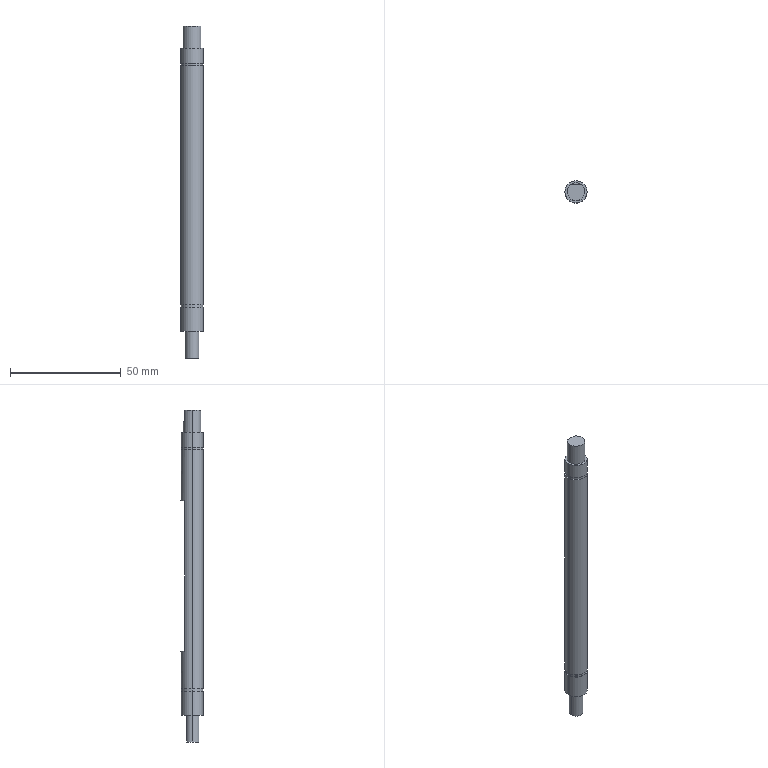Part | SolidWorks | features ICE 4, LibraryFeature 2, RevCut 2, Cut 1, Extrusion 1 | 1 solid | 29 faces | box 10 x 10 x 150 mm | volume 10228 mm3 | cylinder 15 | plane 14 | commonest cylinder face diameters 10 x6 9.6 x4 6.25 x3 8 x2
STEP:
#1=CARTESIAN_POINT('',(5.,0.,65.));
#2=VERTEX_POINT('',#1);
#3=CARTESIAN_POINT('',(-5.,0.,65.));
#4=VERTEX_POINT('',#3);
#5=CARTESIAN_POINT('',(0.,0.,65.));
#6=DIRECTION('',(0.,0.,1.));
#7=DIRECTION('',(1.,0.,0.));
#8=AXIS2_PLACEMENT_3D('',#5,#6,#7);
#9=CIRCLE('',#8,5.);
#10=EDGE_CURVE('',#2,#4,#9,.T.);
#11=ORIENTED_EDGE('',*,*,#10,.F.);
#12=CARTESIAN_POINT('',(5.,0.,58.1));
#13=VERTEX_POINT('',#12);
#14=CARTESIAN_POINT('',(5.,0.,75.));
#15=DIRECTION('',(0.,0.,-1.));
#16=VECTOR('',#15,1000.);
#17=LINE('',#14,#16);
#18=EDGE_CURVE('',#2,#13,#17,.T.);
#19=ORIENTED_EDGE('',*,*,#18,.T.);
#20=CARTESIAN_POINT('',(-5.,0.,58.1));
#21=VERTEX_POINT('',#20);
#22=CARTESIAN_POINT('',(0.,0.,58.1));
#23=DIRECTION('',(0.,0.,1.));
#24=DIRECTION('',(1.,0.,0.));
#25=AXIS2_PLACEMENT_3D('',#22,#23,#24);
#26=CIRCLE('',#25,5.);
#27=EDGE_CURVE('',#13,#21,#26,.T.);
#28=ORIENTED_EDGE('',*,*,#27,.T.);
#29=CARTESIAN_POINT('',(-5.,0.,75.));
#30=DIRECTION('',(0.,0.,-1.));
#31=VECTOR('',#30,1000.);
#32=LINE('',#29,#31);
#33=EDGE_CURVE('',#4,#21,#32,.T.);
#34=ORIENTED_EDGE('',*,*,#33,.F.);
#35=EDGE_LOOP('',(#11,#19,#28,#34));
#36=FACE_OUTER_BOUND('',#35,.T.);
#37=CARTESIAN_POINT('',(0.,0.,75.));
#38=DIRECTION('',(0.,0.,-1.));
#39=DIRECTION('',(-1.,0.,0.));
#40=AXIS2_PLACEMENT_3D('',#37,#38,#39);
#41=CYLINDRICAL_SURFACE('',#40,5.);
#42=ADVANCED_FACE('',(#36),#41,.T.);
#43=CARTESIAN_POINT('',(4.,0.,65.));
#44=VERTEX_POINT('',#43);
#45=CARTESIAN_POINT('',(-4.,0.,65.));
#46=VERTEX_POINT('',#45);
#47=CARTESIAN_POINT('',(0.,0.,65.));
#48=DIRECTION('',(0.,0.,1.));
#49=DIRECTION('',(1.,0.,0.));
#50=AXIS2_PLACEMENT_3D('',#47,#48,#49);
#51=CIRCLE('',#50,4.);
#52=EDGE_CURVE('',#44,#46,#51,.T.);
#53=ORIENTED_EDGE('',*,*,#52,.T.);
#54=CARTESIAN_POINT('',(-4.,0.,75.));
#55=VERTEX_POINT('',#54);
#56=CARTESIAN_POINT('',(-4.,0.,65.));
#57=DIRECTION('',(0.,0.,1.));
#58=VECTOR('',#57,1000.);
#59=LINE('',#56,#58);
#60=EDGE_CURVE('',#46,#55,#59,.T.);
#61=ORIENTED_EDGE('',*,*,#60,.T.);
#62=CARTESIAN_POINT('',(-2.169,3.361,75.));
#63=VERTEX_POINT('',#62);
#64=CARTESIAN_POINT('',(0.,0.,75.));
#65=DIRECTION('',(0.,0.,1.));
#66=DIRECTION('',(1.,0.,0.));
#67=AXIS2_PLACEMENT_3D('',#64,#65,#66);
#68=CIRCLE('',#67,4.);
#69=EDGE_CURVE('',#63,#55,#68,.T.);
#70=ORIENTED_EDGE('',*,*,#69,.F.);
#71=CARTESIAN_POINT('',(-2.169,3.361,70.));
#72=VERTEX_POINT('',#71);
#73=CARTESIAN_POINT('',(-2.169,3.361,65.));
#74=DIRECTION('',(0.,0.,1.));
#75=VECTOR('',#74,1000.);
#76=LINE('',#73,#75);
#77=EDGE_CURVE('',#72,#63,#76,.T.);
#78=ORIENTED_EDGE('',*,*,#77,.F.);
#79=CARTESIAN_POINT('',(2.169,3.361,70.));
#80=VERTEX_POINT('',#79);
#81=CARTESIAN_POINT('',(0.,0.,70.));
#82=DIRECTION('',(0.,0.,-1.));
#83=DIRECTION('',(1.,0.,0.));
#84=AXIS2_PLACEMENT_3D('',#81,#82,#83);
#85=CIRCLE('',#84,4.);
#86=EDGE_CURVE('',#72,#80,#85,.T.);
#87=ORIENTED_EDGE('',*,*,#86,.T.);
#88=CARTESIAN_POINT('',(2.169,3.361,75.));
#89=VERTEX_POINT('',#88);
#90=CARTESIAN_POINT('',(2.169,3.361,65.));
#91=DIRECTION('',(0.,0.,-1.));
#92=VECTOR('',#91,1000.);
#93=LINE('',#90,#92);
#94=EDGE_CURVE('',#89,#80,#93,.T.);
#95=ORIENTED_EDGE('',*,*,#94,.F.);
#96=CARTESIAN_POINT('',(4.,0.,75.));
#97=VERTEX_POINT('',#96);
#98=CARTESIAN_POINT('',(0.,0.,75.));
#99=DIRECTION('',(0.,0.,1.));
#100=DIRECTION('',(1.,0.,0.));
#101=AXIS2_PLACEMENT_3D('',#98,#99,#100);
#102=CIRCLE('',#101,4.);
#103=EDGE_CURVE('',#97,#89,#102,.T.);
#104=ORIENTED_EDGE('',*,*,#103,.F.);
#105=CARTESIAN_POINT('',(4.,0.,65.));
#106=DIRECTION('',(0.,0.,1.));
#107=VECTOR('',#106,1000.);
#108=LINE('',#105,#107);
#109=EDGE_CURVE('',#44,#97,#108,.T.);
#110=ORIENTED_EDGE('',*,*,#109,.F.);
#111=EDGE_LOOP('',(#53,#61,#70,#78,#87,#95,#104,#110));
#112=FACE_OUTER_BOUND('',#111,.T.);
#113=CARTESIAN_POINT('',(0.,0.,65.));
#114=DIRECTION('',(0.,0.,1.));
#115=DIRECTION('',(1.,0.,0.));
#116=AXIS2_PLACEMENT_3D('',#113,#114,#115);
#117=CYLINDRICAL_SURFACE('',#116,4.);
#118=ADVANCED_FACE('',(#112),#117,.T.);
#119=CARTESIAN_POINT('',(4.8,0.,57.));
#120=VERTEX_POINT('',#119);
#121=CARTESIAN_POINT('',(-4.8,0.,57.));
#122=VERTEX_POINT('',#121);
#123=CARTESIAN_POINT('',(0.,0.,57.));
#124=DIRECTION('',(0.,0.,1.));
#125=DIRECTION('',(1.,0.,0.));
#126=AXIS2_PLACEMENT_3D('',#123,#124,#125);
#127=CIRCLE('',#126,4.8);
#128=EDGE_CURVE('',#120,#122,#127,.T.);
#129=ORIENTED_EDGE('',*,*,#128,.T.);
#130=CARTESIAN_POINT('',(-4.8,0.,58.1));
#131=VERTEX_POINT('',#130);
#132=CARTESIAN_POINT('',(-4.8,0.,65.));
#133=DIRECTION('',(0.,0.,1.));
#134=VECTOR('',#133,1000.);
#135=LINE('',#132,#134);
#136=EDGE_CURVE('',#122,#131,#135,.T.);
#137=ORIENTED_EDGE('',*,*,#136,.T.);
#138=CARTESIAN_POINT('',(4.8,0.,58.1));
#139=VERTEX_POINT('',#138);
#140=CARTESIAN_POINT('',(0.,0.,58.1));
#141=DIRECTION('',(0.,0.,1.));
#142=DIRECTION('',(1.,0.,0.));
#143=AXIS2_PLACEMENT_3D('',#140,#141,#142);
#144=CIRCLE('',#143,4.8);
#145=EDGE_CURVE('',#139,#131,#144,.T.);
#146=ORIENTED_EDGE('',*,*,#145,.F.);
#147=CARTESIAN_POINT('',(4.8,0.,65.));
#148=DIRECTION('',(0.,0.,1.));
#149=VECTOR('',#148,1000.);
#150=LINE('',#147,#149);
#151=EDGE_CURVE('',#120,#139,#150,.T.);
#152=ORIENTED_EDGE('',*,*,#151,.F.);
#153=EDGE_LOOP('',(#129,#137,#146,#152));
#154=FACE_OUTER_BOUND('',#153,.T.);
#155=CARTESIAN_POINT('',(0.,0.,65.));
#156=DIRECTION('',(0.,0.,1.));
#157=DIRECTION('',(1.,0.,0.));
#158=AXIS2_PLACEMENT_3D('',#155,#156,#157);
#159=CYLINDRICAL_SURFACE('',#158,4.8);
#160=ADVANCED_FACE('',(#154),#159,.T.);
#161=CARTESIAN_POINT('',(3.842,3.2,34.));
#162=VERTEX_POINT('',#161);
#163=CARTESIAN_POINT('',(-3.842,3.2,34.));
#164=VERTEX_POINT('',#163);
#165=CARTESIAN_POINT('',(0.,0.,34.));
#166=DIRECTION('',(0.,0.,1.));
#167=DIRECTION('',(1.,0.,0.));
#168=AXIS2_PLACEMENT_3D('',#165,#166,#167);
#169=CIRCLE('',#168,5.);
#170=EDGE_CURVE('',#162,#164,#169,.T.);
#171=ORIENTED_EDGE('',*,*,#170,.T.);
#172=CARTESIAN_POINT('',(-3.842,3.2,-34.));
#173=VERTEX_POINT('',#172);
#174=CARTESIAN_POINT('',(-3.842,3.2,75.));
#175=DIRECTION('',(0.,0.,-1.));
#176=VECTOR('',#175,1000.);
#177=LINE('',#174,#176);
#178=EDGE_CURVE('',#164,#173,#177,.T.);
#179=ORIENTED_EDGE('',*,*,#178,.T.);
#180=CARTESIAN_POINT('',(3.842,3.2,-34.));
#181=VERTEX_POINT('',#180);
#182=CARTESIAN_POINT('',(0.,0.,-34.));
#183=DIRECTION('',(0.,0.,-1.));
#184=DIRECTION('',(-1.,0.,0.));
#185=AXIS2_PLACEMENT_3D('',#182,#183,#184);
#186=CIRCLE('',#185,5.);
#187=EDGE_CURVE('',#173,#181,#186,.T.);
#188=ORIENTED_EDGE('',*,*,#187,.T.);
#189=CARTESIAN_POINT('',(3.842,3.2,75.));
#190=DIRECTION('',(0.,0.,1.));
#191=VECTOR('',#190,1000.);
#192=LINE('',#189,#191);
#193=EDGE_CURVE('',#181,#162,#192,.T.);
#194=ORIENTED_EDGE('',*,*,#193,.T.);
#195=EDGE_LOOP('',(#171,#179,#188,#194));
#196=FACE_BOUND('',#195,.T.);
#197=CARTESIAN_POINT('',(5.,0.,57.));
#198=VERTEX_POINT('',#197);
#199=CARTESIAN_POINT('',(-5.,0.,57.));
#200=VERTEX_POINT('',#199);
#201=CARTESIAN_POINT('',(0.,0.,57.));
#202=DIRECTION('',(0.,0.,1.));
#203=DIRECTION('',(1.,0.,0.));
#204=AXIS2_PLACEMENT_3D('',#201,#202,#203);
#205=CIRCLE('',#204,5.);
#206=EDGE_CURVE('',#198,#200,#205,.T.);
#207=ORIENTED_EDGE('',*,*,#206,.F.);
#208=CARTESIAN_POINT('',(5.,0.,-51.));
#209=VERTEX_POINT('',#208);
#210=CARTESIAN_POINT('',(5.,0.,75.));
#211=DIRECTION('',(0.,0.,-1.));
#212=VECTOR('',#211,1000.);
#213=LINE('',#210,#212);
#214=EDGE_CURVE('',#198,#209,#213,.T.);
#215=ORIENTED_EDGE('',*,*,#214,.T.);
#216=CARTESIAN_POINT('',(-5.,0.,-51.));
#217=VERTEX_POINT('',#216);
#218=CARTESIAN_POINT('',(0.,0.,-51.));
#219=DIRECTION('',(0.,0.,-1.));
#220=DIRECTION('',(-1.,0.,0.));
#221=AXIS2_PLACEMENT_3D('',#218,#219,#220);
#222=CIRCLE('',#221,5.);
#223=EDGE_CURVE('',#217,#209,#222,.T.);
#224=ORIENTED_EDGE('',*,*,#223,.F.);
#225=CARTESIAN_POINT('',(-5.,0.,75.));
#226=DIRECTION('',(0.,0.,-1.));
#227=VECTOR('',#226,1000.);
#228=LINE('',#225,#227);
#229=EDGE_CURVE('',#200,#217,#228,.T.);
#230=ORIENTED_EDGE('',*,*,#229,.F.);
#231=EDGE_LOOP('',(#207,#215,#224,#230));
#232=FACE_OUTER_BOUND('',#231,.T.);
#233=CARTESIAN_POINT('',(0.,0.,75.));
#234=DIRECTION('',(0.,0.,-1.));
#235=DIRECTION('',(-1.,0.,0.));
#236=AXIS2_PLACEMENT_3D('',#233,#234,#235);
#237=CYLINDRICAL_SURFACE('',#236,5.);
#238=ADVANCED_FACE('',(#196,#232),#237,.T.);
#239=CARTESIAN_POINT('',(-4.8,0.,-51.));
#240=VERTEX_POINT('',#239);
#241=CARTESIAN_POINT('',(4.8,0.,-51.));
#242=VERTEX_POINT('',#241);
#243=CARTESIAN_POINT('',(0.,0.,-51.));
#244=DIRECTION('',(0.,0.,-1.));
#245=DIRECTION('',(-1.,0.,0.));
#246=AXIS2_PLACEMENT_3D('',#243,#244,#245);
#247=CIRCLE('',#246,4.8);
#248=EDGE_CURVE('',#240,#242,#247,.T.);
#249=ORIENTED_EDGE('',*,*,#248,.T.);
#250=CARTESIAN_POINT('',(4.8,0.,-52.1));
#251=VERTEX_POINT('',#250);
#252=CARTESIAN_POINT('',(4.8,0.,-63.));
#253=DIRECTION('',(0.,0.,-1.));
#254=VECTOR('',#253,1000.);
#255=LINE('',#252,#254);
#256=EDGE_CURVE('',#242,#251,#255,.T.);
#257=ORIENTED_EDGE('',*,*,#256,.T.);
#258=CARTESIAN_POINT('',(-4.8,0.,-52.1));
#259=VERTEX_POINT('',#258);
#260=CARTESIAN_POINT('',(0.,0.,-52.1));
#261=DIRECTION('',(0.,0.,-1.));
#262=DIRECTION('',(-1.,0.,0.));
#263=AXIS2_PLACEMENT_3D('',#260,#261,#262);
#264=CIRCLE('',#263,4.8);
#265=EDGE_CURVE('',#259,#251,#264,.T.);
#266=ORIENTED_EDGE('',*,*,#265,.F.);
#267=CARTESIAN_POINT('',(-4.8,0.,-63.));
#268=DIRECTION('',(0.,0.,-1.));
#269=VECTOR('',#268,1000.);
#270=LINE('',#267,#269);
#271=EDGE_CURVE('',#240,#259,#270,.T.);
#272=ORIENTED_EDGE('',*,*,#271,.F.);
#273=EDGE_LOOP('',(#249,#257,#266,#272));
#274=FACE_OUTER_BOUND('',#273,.T.);
#275=CARTESIAN_POINT('',(0.,0.,-63.));
#276=DIRECTION('',(0.,0.,-1.));
#277=DIRECTION('',(-1.,0.,0.));
#278=AXIS2_PLACEMENT_3D('',#275,#276,#277);
#279=CYLINDRICAL_SURFACE('',#278,4.8);
#280=ADVANCED_FACE('',(#274),#279,.T.);
#281=CARTESIAN_POINT('',(1.875,2.5,-63.));
#282=VERTEX_POINT('',#281);
#283=CARTESIAN_POINT('',(3.125,0.,-63.));
#284=VERTEX_POINT('',#283);
#285=CARTESIAN_POINT('',(0.,0.,-63.));
#286=DIRECTION('',(0.,0.,-1.));
#287=DIRECTION('',(-1.,0.,0.));
#288=AXIS2_PLACEMENT_3D('',#285,#286,#287);
#289=CIRCLE('',#288,3.125);
#290=EDGE_CURVE('',#282,#284,#289,.T.);
#291=ORIENTED_EDGE('',*,*,#290,.T.);
#292=CARTESIAN_POINT('',(3.125,0.,-75.));
#293=VERTEX_POINT('',#292);
#294=CARTESIAN_POINT('',(3.125,0.,-63.));
#295=DIRECTION('',(0.,0.,-1.));
#296=VECTOR('',#295,1000.);
#297=LINE('',#294,#296);
#298=EDGE_CURVE('',#284,#293,#297,.T.);
#299=ORIENTED_EDGE('',*,*,#298,.T.);
#300=CARTESIAN_POINT('',(1.875,2.5,-75.));
#301=VERTEX_POINT('',#300);
#302=CARTESIAN_POINT('',(0.,0.,-75.));
#303=DIRECTION('',(0.,0.,-1.));
#304=DIRECTION('',(-1.,0.,0.));
#305=AXIS2_PLACEMENT_3D('',#302,#303,#304);
#306=CIRCLE('',#305,3.125);
#307=EDGE_CURVE('',#301,#293,#306,.T.);
#308=ORIENTED_EDGE('',*,*,#307,.F.);
#309=CARTESIAN_POINT('',(1.875,2.5,-63.));
#310=DIRECTION('',(0.,0.,1.));
#311=VECTOR('',#310,1000.);
#312=LINE('',#309,#311);
#313=EDGE_CURVE('',#301,#282,#312,.T.);
#314=ORIENTED_EDGE('',*,*,#313,.T.);
#315=EDGE_LOOP('',(#291,#299,#308,#314));
#316=FACE_OUTER_BOUND('',#315,.T.);
#317=CARTESIAN_POINT('',(0.,0.,-63.));
#318=DIRECTION('',(0.,0.,-1.));
#319=DIRECTION('',(-1.,0.,0.));
#320=AXIS2_PLACEMENT_3D('',#317,#318,#319);
#321=CYLINDRICAL_SURFACE('',#320,3.125);
#322=ADVANCED_FACE('',(#316),#321,.T.);
#323=ORIENTED_EDGE('',*,*,#298,.F.);
#324=CARTESIAN_POINT('',(-3.125,0.,-63.));
#325=VERTEX_POINT('',#324);
#326=CARTESIAN_POINT('',(0.,0.,-63.));
#327=DIRECTION('',(0.,0.,-1.));
#328=DIRECTION('',(-1.,0.,0.));
#329=AXIS2_PLACEMENT_3D('',#326,#327,#328);
#330=CIRCLE('',#329,3.125);
#331=EDGE_CURVE('',#284,#325,#330,.T.);
#332=ORIENTED_EDGE('',*,*,#331,.T.);
#333=CARTESIAN_POINT('',(-3.125,0.,-75.));
#334=VERTEX_POINT('',#333);
#335=CARTESIAN_POINT('',(-3.125,0.,-63.));
#336=DIRECTION('',(0.,0.,-1.));
#337=VECTOR('',#336,1000.);
#338=LINE('',#335,#337);
#339=EDGE_CURVE('',#325,#334,#338,.T.);
#340=ORIENTED_EDGE('',*,*,#339,.T.);
#341=CARTESIAN_POINT('',(0.,0.,-75.));
#342=DIRECTION('',(0.,0.,-1.));
#343=DIRECTION('',(-1.,0.,0.));
#344=AXIS2_PLACEMENT_3D('',#341,#342,#343);
#345=CIRCLE('',#344,3.125);
#346=EDGE_CURVE('',#293,#334,#345,.T.);
#347=ORIENTED_EDGE('',*,*,#346,.F.);
#348=EDGE_LOOP('',(#323,#332,#340,#347));
#349=FACE_OUTER_BOUND('',#348,.T.);
#350=CARTESIAN_POINT('',(0.,0.,-63.));
#351=DIRECTION('',(0.,0.,-1.));
#352=DIRECTION('',(-1.,0.,0.));
#353=AXIS2_PLACEMENT_3D('',#350,#351,#352);
#354=CYLINDRICAL_SURFACE('',#353,3.125);
#355=ADVANCED_FACE('',(#349),#354,.T.);
#356=CARTESIAN_POINT('',(-5.,0.,-52.1));
#357=VERTEX_POINT('',#356);
#358=CARTESIAN_POINT('',(5.,0.,-52.1));
#359=VERTEX_POINT('',#358);
#360=CARTESIAN_POINT('',(0.,0.,-52.1));
#361=DIRECTION('',(0.,0.,-1.));
#362=DIRECTION('',(-1.,0.,0.));
#363=AXIS2_PLACEMENT_3D('',#360,#361,#362);
#364=CIRCLE('',#363,5.);
#365=EDGE_CURVE('',#357,#359,#364,.T.);
#366=ORIENTED_EDGE('',*,*,#365,.T.);
#367=CARTESIAN_POINT('',(5.,0.,-63.));
#368=VERTEX_POINT('',#367);
#369=CARTESIAN_POINT('',(5.,0.,75.));
#370=DIRECTION('',(0.,0.,-1.));
#371=VECTOR('',#370,1000.);
#372=LINE('',#369,#371);
#373=EDGE_CURVE('',#359,#368,#372,.T.);
#374=ORIENTED_EDGE('',*,*,#373,.T.);
#375=CARTESIAN_POINT('',(-5.,0.,-63.));
#376=VERTEX_POINT('',#375);
#377=CARTESIAN_POINT('',(0.,0.,-63.));
#378=DIRECTION('',(0.,0.,-1.));
#379=DIRECTION('',(-1.,0.,0.));
#380=AXIS2_PLACEMENT_3D('',#377,#378,#379);
#381=CIRCLE('',#380,5.);
#382=EDGE_CURVE('',#376,#368,#381,.T.);
#383=ORIENTED_EDGE('',*,*,#382,.F.);
#384=CARTESIAN_POINT('',(-5.,0.,75.));
#385=DIRECTION('',(0.,0.,-1.));
#386=VECTOR('',#385,1000.);
#387=LINE('',#384,#386);
#388=EDGE_CURVE('',#357,#376,#387,.T.);
#389=ORIENTED_EDGE('',*,*,#388,.F.);
#390=EDGE_LOOP('',(#366,#374,#383,#389));
#391=FACE_OUTER_BOUND('',#390,.T.);
#392=CARTESIAN_POINT('',(0.,0.,75.));
#393=DIRECTION('',(0.,0.,-1.));
#394=DIRECTION('',(-1.,0.,0.));
#395=AXIS2_PLACEMENT_3D('',#392,#393,#394);
#396=CYLINDRICAL_SURFACE('',#395,5.);
#397=ADVANCED_FACE('',(#391),#396,.T.);
#398=ORIENTED_EDGE('',*,*,#373,.F.);
#399=CARTESIAN_POINT('',(0.,0.,-52.1));
#400=DIRECTION('',(0.,0.,-1.));
#401=DIRECTION('',(-1.,0.,0.));
#402=AXIS2_PLACEMENT_3D('',#399,#400,#401);
#403=CIRCLE('',#402,5.);
#404=EDGE_CURVE('',#359,#357,#403,.T.);
#405=ORIENTED_EDGE('',*,*,#404,.T.);
#406=ORIENTED_EDGE('',*,*,#388,.T.);
#407=CARTESIAN_POINT('',(0.,0.,-63.));
#408=DIRECTION('',(0.,0.,-1.));
#409=DIRECTION('',(-1.,0.,0.));
#410=AXIS2_PLACEMENT_3D('',#407,#408,#409);
#411=CIRCLE('',#410,5.);
#412=EDGE_CURVE('',#368,#376,#411,.T.);
#413=ORIENTED_EDGE('',*,*,#412,.F.);
#414=EDGE_LOOP('',(#398,#405,#406,#413));
#415=FACE_OUTER_BOUND('',#414,.T.);
#416=CARTESIAN_POINT('',(0.,0.,75.));
#417=DIRECTION('',(0.,0.,-1.));
#418=DIRECTION('',(-1.,0.,0.));
#419=AXIS2_PLACEMENT_3D('',#416,#417,#418);
#420=CYLINDRICAL_SURFACE('',#419,5.);
#421=ADVANCED_FACE('',(#415),#420,.T.);
#422=ORIENTED_EDGE('',*,*,#339,.F.);
#423=CARTESIAN_POINT('',(-1.875,2.5,-63.));
#424=VERTEX_POINT('',#423);
#425=CARTESIAN_POINT('',(0.,0.,-63.));
#426=DIRECTION('',(0.,0.,-1.));
#427=DIRECTION('',(-1.,0.,0.));
#428=AXIS2_PLACEMENT_3D('',#425,#426,#427);
#429=CIRCLE('',#428,3.125);
#430=EDGE_CURVE('',#325,#424,#429,.T.);
#431=ORIENTED_EDGE('',*,*,#430,.T.);
#432=CARTESIAN_POINT('',(-1.875,2.5,-75.));
#433=VERTEX_POINT('',#432);
#434=CARTESIAN_POINT('',(-1.875,2.5,-63.));
#435=DIRECTION('',(0.,0.,-1.));
#436=VECTOR('',#435,1000.);
#437=LINE('',#434,#436);
#438=EDGE_CURVE('',#424,#433,#437,.T.);
#439=ORIENTED_EDGE('',*,*,#438,.T.);
#440=CARTESIAN_POINT('',(0.,0.,-75.));
#441=DIRECTION('',(0.,0.,-1.));
#442=DIRECTION('',(-1.,0.,0.));
#443=AXIS2_PLACEMENT_3D('',#440,#441,#442);
#444=CIRCLE('',#443,3.125);
#445=EDGE_CURVE('',#334,#433,#444,.T.);
#446=ORIENTED_EDGE('',*,*,#445,.F.);
#447=EDGE_LOOP('',(#422,#431,#439,#446));
#448=FACE_OUTER_BOUND('',#447,.T.);
#449=CARTESIAN_POINT('',(0.,0.,-63.));
#450=DIRECTION('',(0.,0.,-1.));
#451=DIRECTION('',(-1.,0.,0.));
#452=AXIS2_PLACEMENT_3D('',#449,#450,#451);
#453=CYLINDRICAL_SURFACE('',#452,3.125);
#454=ADVANCED_FACE('',(#448),#453,.T.);
#455=CARTESIAN_POINT('',(0.,2.5,-75.));
#456=DIRECTION('',(-1.,0.,0.));
#457=VECTOR('',#456,1000.);
#458=LINE('',#455,#457);
#459=EDGE_CURVE('',#301,#433,#458,.T.);
#460=ORIENTED_EDGE('',*,*,#459,.F.);
#461=ORIENTED_EDGE('',*,*,#307,.T.);
#462=ORIENTED_EDGE('',*,*,#346,.T.);
#463=ORIENTED_EDGE('',*,*,#445,.T.);
#464=EDGE_LOOP('',(#460,#461,#462,#463));
#465=FACE_OUTER_BOUND('',#464,.T.);
#466=CARTESIAN_POINT('',(0.,0.,-75.));
#467=DIRECTION('',(0.,0.,1.));
#468=DIRECTION('',(1.,0.,0.));
#469=AXIS2_PLACEMENT_3D('',#466,#467,#468);
#470=PLANE('',#469);
#471=ADVANCED_FACE('',(#465),#470,.F.);
#472=CARTESIAN_POINT('',(1.957,2.5,-63.));
#473=DIRECTION('',(1.,0.,0.));
#474=VECTOR('',#473,1000.);
#475=LINE('',#472,#474);
#476=EDGE_CURVE('',#424,#282,#475,.T.);
#477=ORIENTED_EDGE('',*,*,#476,.F.);
#478=ORIENTED_EDGE('',*,*,#430,.F.);
#479=ORIENTED_EDGE('',*,*,#331,.F.);
#480=ORIENTED_EDGE('',*,*,#290,.F.);
#481=EDGE_LOOP('',(#477,#478,#479,#480));
#482=FACE_BOUND('',#481,.T.);
#483=ORIENTED_EDGE('',*,*,#382,.T.);
#484=ORIENTED_EDGE('',*,*,#412,.T.);
#485=EDGE_LOOP('',(#483,#484));
#486=FACE_OUTER_BOUND('',#485,.T.);
#487=CARTESIAN_POINT('',(0.,0.,-63.));
#488=DIRECTION('',(0.,0.,-1.));
#489=DIRECTION('',(-1.,0.,0.));
#490=AXIS2_PLACEMENT_3D('',#487,#488,#489);
#491=PLANE('',#490);
#492=ADVANCED_FACE('',(#482,#486),#491,.T.);
#493=ORIENTED_EDGE('',*,*,#459,.T.);
#494=ORIENTED_EDGE('',*,*,#438,.F.);
#495=ORIENTED_EDGE('',*,*,#476,.T.);
#496=ORIENTED_EDGE('',*,*,#313,.F.);
#497=EDGE_LOOP('',(#493,#494,#495,#496));
#498=FACE_OUTER_BOUND('',#497,.T.);
#499=CARTESIAN_POINT('',(1.957,2.5,-63.));
#500=DIRECTION('',(0.,1.,0.));
#501=DIRECTION('',(0.,0.,1.));
#502=AXIS2_PLACEMENT_3D('',#499,#500,#501);
#503=PLANE('',#502);
#504=ADVANCED_FACE('',(#498),#503,.T.);
#505=ORIENTED_EDGE('',*,*,#365,.F.);
#506=ORIENTED_EDGE('',*,*,#404,.F.);
#507=EDGE_LOOP('',(#505,#506));
#508=FACE_OUTER_BOUND('',#507,.T.);
#509=ORIENTED_EDGE('',*,*,#265,.T.);
#510=CARTESIAN_POINT('',(0.,0.,-52.1));
#511=DIRECTION('',(0.,0.,-1.));
#512=DIRECTION('',(-1.,0.,0.));
#513=AXIS2_PLACEMENT_3D('',#510,#511,#512);
#514=CIRCLE('',#513,4.8);
#515=EDGE_CURVE('',#251,#259,#514,.T.);
#516=ORIENTED_EDGE('',*,*,#515,.T.);
#517=EDGE_LOOP('',(#509,#516));
#518=FACE_BOUND('',#517,.T.);
#519=CARTESIAN_POINT('',(-5.,0.,-52.1));
#520=DIRECTION('',(0.,0.,-1.));
#521=DIRECTION('',(-1.,0.,0.));
#522=AXIS2_PLACEMENT_3D('',#519,#520,#521);
#523=PLANE('',#522);
#524=ADVANCED_FACE('',(#508,#518),#523,.F.);
#525=ORIENTED_EDGE('',*,*,#256,.F.);
#526=CARTESIAN_POINT('',(0.,0.,-51.));
#527=DIRECTION('',(0.,0.,-1.));
#528=DIRECTION('',(-1.,0.,0.));
#529=AXIS2_PLACEMENT_3D('',#526,#527,#528);
#530=CIRCLE('',#529,4.8);
#531=EDGE_CURVE('',#242,#240,#530,.T.);
#532=ORIENTED_EDGE('',*,*,#531,.T.);
#533=ORIENTED_EDGE('',*,*,#271,.T.);
#534=ORIENTED_EDGE('',*,*,#515,.F.);
#535=EDGE_LOOP('',(#525,#532,#533,#534));
#536=FACE_OUTER_BOUND('',#535,.T.);
#537=CARTESIAN_POINT('',(0.,0.,-63.));
#538=DIRECTION('',(0.,0.,-1.));
#539=DIRECTION('',(-1.,0.,0.));
#540=AXIS2_PLACEMENT_3D('',#537,#538,#539);
#541=CYLINDRICAL_SURFACE('',#540,4.8);
#542=ADVANCED_FACE('',(#536),#541,.T.);
#543=ORIENTED_EDGE('',*,*,#248,.F.);
#544=ORIENTED_EDGE('',*,*,#531,.F.);
#545=EDGE_LOOP('',(#543,#544));
#546=FACE_BOUND('',#545,.T.);
#547=ORIENTED_EDGE('',*,*,#223,.T.);
#548=CARTESIAN_POINT('',(0.,0.,-51.));
#549=DIRECTION('',(0.,0.,-1.));
#550=DIRECTION('',(-1.,0.,0.));
#551=AXIS2_PLACEMENT_3D('',#548,#549,#550);
#552=CIRCLE('',#551,5.);
#553=EDGE_CURVE('',#209,#217,#552,.T.);
#554=ORIENTED_EDGE('',*,*,#553,.T.);
#555=EDGE_LOOP('',(#547,#554));
#556=FACE_OUTER_BOUND('',#555,.T.);
#557=CARTESIAN_POINT('',(-5.,0.,-51.));
#558=DIRECTION('',(0.,0.,1.));
#559=DIRECTION('',(1.,0.,0.));
#560=AXIS2_PLACEMENT_3D('',#557,#558,#559);
#561=PLANE('',#560);
#562=ADVANCED_FACE('',(#546,#556),#561,.F.);
#563=CARTESIAN_POINT('',(-5.,3.2,-34.));
#564=DIRECTION('',(1.,0.,0.));
#565=VECTOR('',#564,1000.);
#566=LINE('',#563,#565);
#567=EDGE_CURVE('',#173,#181,#566,.T.);
#568=ORIENTED_EDGE('',*,*,#567,.T.);
#569=ORIENTED_EDGE('',*,*,#187,.F.);
#570=EDGE_LOOP('',(#568,#569));
#571=FACE_OUTER_BOUND('',#570,.T.);
#572=CARTESIAN_POINT('',(-5.,17.735,-34.));
#573=DIRECTION('',(0.,0.,-1.));
#574=DIRECTION('',(-1.,0.,0.));
#575=AXIS2_PLACEMENT_3D('',#572,#573,#574);
#576=PLANE('',#575);
#577=ADVANCED_FACE('',(#571),#576,.F.);
#578=CARTESIAN_POINT('',(-5.,3.2,34.));
#579=DIRECTION('',(1.,0.,0.));
#580=VECTOR('',#579,1000.);
#581=LINE('',#578,#580);
#582=EDGE_CURVE('',#164,#162,#581,.T.);
#583=ORIENTED_EDGE('',*,*,#582,.T.);
#584=ORIENTED_EDGE('',*,*,#193,.F.);
#585=ORIENTED_EDGE('',*,*,#567,.F.);
#586=ORIENTED_EDGE('',*,*,#178,.F.);
#587=EDGE_LOOP('',(#583,#584,#585,#586));
#588=FACE_OUTER_BOUND('',#587,.T.);
#589=CARTESIAN_POINT('',(-5.,3.2,34.));
#590=DIRECTION('',(0.,-1.,0.));
#591=DIRECTION('',(0.,0.,-1.));
#592=AXIS2_PLACEMENT_3D('',#589,#590,#591);
#593=PLANE('',#592);
#594=ADVANCED_FACE('',(#588),#593,.F.);
#595=ORIENTED_EDGE('',*,*,#582,.F.);
#596=ORIENTED_EDGE('',*,*,#170,.F.);
#597=EDGE_LOOP('',(#595,#596));
#598=FACE_OUTER_BOUND('',#597,.T.);
#599=CARTESIAN_POINT('',(-5.,17.735,34.));
#600=DIRECTION('',(0.,0.,1.));
#601=DIRECTION('',(1.,0.,0.));
#602=AXIS2_PLACEMENT_3D('',#599,#600,#601);
#603=PLANE('',#602);
#604=ADVANCED_FACE('',(#598),#603,.F.);
#605=ORIENTED_EDGE('',*,*,#214,.F.);
#606=CARTESIAN_POINT('',(0.,0.,57.));
#607=DIRECTION('',(0.,0.,1.));
#608=DIRECTION('',(1.,0.,0.));
#609=AXIS2_PLACEMENT_3D('',#606,#607,#608);
#610=CIRCLE('',#609,5.);
#611=EDGE_CURVE('',#200,#198,#610,.T.);
#612=ORIENTED_EDGE('',*,*,#611,.F.);
#613=ORIENTED_EDGE('',*,*,#229,.T.);
#614=ORIENTED_EDGE('',*,*,#553,.F.);
#615=EDGE_LOOP('',(#605,#612,#613,#614));
#616=FACE_OUTER_BOUND('',#615,.T.);
#617=CARTESIAN_POINT('',(0.,0.,75.));
#618=DIRECTION('',(0.,0.,-1.));
#619=DIRECTION('',(-1.,0.,0.));
#620=AXIS2_PLACEMENT_3D('',#617,#618,#619);
#621=CYLINDRICAL_SURFACE('',#620,5.);
#622=ADVANCED_FACE('',(#616),#621,.T.);
#623=CARTESIAN_POINT('',(0.,0.,58.1));
#624=DIRECTION('',(0.,0.,1.));
#625=DIRECTION('',(1.,0.,0.));
#626=AXIS2_PLACEMENT_3D('',#623,#624,#625);
#627=CIRCLE('',#626,5.);
#628=EDGE_CURVE('',#21,#13,#627,.T.);
#629=ORIENTED_EDGE('',*,*,#628,.F.);
#630=ORIENTED_EDGE('',*,*,#27,.F.);
#631=EDGE_LOOP('',(#629,#630));
#632=FACE_OUTER_BOUND('',#631,.T.);
#633=ORIENTED_EDGE('',*,*,#145,.T.);
#634=CARTESIAN_POINT('',(0.,0.,58.1));
#635=DIRECTION('',(0.,0.,1.));
#636=DIRECTION('',(1.,0.,0.));
#637=AXIS2_PLACEMENT_3D('',#634,#635,#636);
#638=CIRCLE('',#637,4.8);
#639=EDGE_CURVE('',#131,#139,#638,.T.);
#640=ORIENTED_EDGE('',*,*,#639,.T.);
#641=EDGE_LOOP('',(#633,#640));
#642=FACE_BOUND('',#641,.T.);
#643=CARTESIAN_POINT('',(5.,0.,58.1));
#644=DIRECTION('',(0.,0.,1.));
#645=DIRECTION('',(1.,0.,0.));
#646=AXIS2_PLACEMENT_3D('',#643,#644,#645);
#647=PLANE('',#646);
#648=ADVANCED_FACE('',(#632,#642),#647,.F.);
#649=ORIENTED_EDGE('',*,*,#136,.F.);
#650=CARTESIAN_POINT('',(0.,0.,57.));
#651=DIRECTION('',(0.,0.,1.));
#652=DIRECTION('',(1.,0.,0.));
#653=AXIS2_PLACEMENT_3D('',#650,#651,#652);
#654=CIRCLE('',#653,4.8);
#655=EDGE_CURVE('',#122,#120,#654,.T.);
#656=ORIENTED_EDGE('',*,*,#655,.T.);
#657=ORIENTED_EDGE('',*,*,#151,.T.);
#658=ORIENTED_EDGE('',*,*,#639,.F.);
#659=EDGE_LOOP('',(#649,#656,#657,#658));
#660=FACE_OUTER_BOUND('',#659,.T.);
#661=CARTESIAN_POINT('',(0.,0.,65.));
#662=DIRECTION('',(0.,0.,1.));
#663=DIRECTION('',(1.,0.,0.));
#664=AXIS2_PLACEMENT_3D('',#661,#662,#663);
#665=CYLINDRICAL_SURFACE('',#664,4.8);
#666=ADVANCED_FACE('',(#660),#665,.T.);
#667=ORIENTED_EDGE('',*,*,#128,.F.);
#668=ORIENTED_EDGE('',*,*,#655,.F.);
#669=EDGE_LOOP('',(#667,#668));
#670=FACE_BOUND('',#669,.T.);
#671=ORIENTED_EDGE('',*,*,#611,.T.);
#672=ORIENTED_EDGE('',*,*,#206,.T.);
#673=EDGE_LOOP('',(#671,#672));
#674=FACE_OUTER_BOUND('',#673,.T.);
#675=CARTESIAN_POINT('',(5.,0.,57.));
#676=DIRECTION('',(0.,0.,-1.));
#677=DIRECTION('',(-1.,0.,0.));
#678=AXIS2_PLACEMENT_3D('',#675,#676,#677);
#679=PLANE('',#678);
#680=ADVANCED_FACE('',(#670,#674),#679,.F.);
#681=CARTESIAN_POINT('',(-5.016,3.361,70.));
#682=DIRECTION('',(1.,0.,0.));
#683=VECTOR('',#682,1000.);
#684=LINE('',#681,#683);
#685=EDGE_CURVE('',#72,#80,#684,.T.);
#686=ORIENTED_EDGE('',*,*,#685,.T.);
#687=ORIENTED_EDGE('',*,*,#86,.F.);
#688=EDGE_LOOP('',(#686,#687));
#689=FACE_OUTER_BOUND('',#688,.T.);
#690=CARTESIAN_POINT('',(0.,0.,70.));
#691=DIRECTION('',(0.,0.,1.));
#692=DIRECTION('',(1.,0.,0.));
#693=AXIS2_PLACEMENT_3D('',#690,#691,#692);
#694=PLANE('',#693);
#695=ADVANCED_FACE('',(#689),#694,.T.);
#696=CARTESIAN_POINT('',(0.,3.361,75.));
#697=DIRECTION('',(1.,0.,0.));
#698=VECTOR('',#697,1000.);
#699=LINE('',#696,#698);
#700=EDGE_CURVE('',#63,#89,#699,.T.);
#701=ORIENTED_EDGE('',*,*,#700,.F.);
#702=ORIENTED_EDGE('',*,*,#69,.T.);
#703=CARTESIAN_POINT('',(0.,0.,75.));
#704=DIRECTION('',(0.,0.,1.));
#705=DIRECTION('',(1.,0.,0.));
#706=AXIS2_PLACEMENT_3D('',#703,#704,#705);
#707=CIRCLE('',#706,4.);
#708=EDGE_CURVE('',#55,#97,#707,.T.);
#709=ORIENTED_EDGE('',*,*,#708,.T.);
#710=ORIENTED_EDGE('',*,*,#103,.T.);
#711=EDGE_LOOP('',(#701,#702,#709,#710));
#712=FACE_OUTER_BOUND('',#711,.T.);
#713=CARTESIAN_POINT('',(0.,0.,75.));
#714=DIRECTION('',(0.,0.,1.));
#715=DIRECTION('',(1.,0.,0.));
#716=AXIS2_PLACEMENT_3D('',#713,#714,#715);
#717=PLANE('',#716);
#718=ADVANCED_FACE('',(#712),#717,.T.);
#719=ORIENTED_EDGE('',*,*,#94,.T.);
#720=ORIENTED_EDGE('',*,*,#685,.F.);
#721=ORIENTED_EDGE('',*,*,#77,.T.);
#722=ORIENTED_EDGE('',*,*,#700,.T.);
#723=EDGE_LOOP('',(#719,#720,#721,#722));
#724=FACE_OUTER_BOUND('',#723,.T.);
#725=CARTESIAN_POINT('',(-5.016,3.361,70.));
#726=DIRECTION('',(0.,-1.,0.));
#727=DIRECTION('',(0.,0.,-1.));
#728=AXIS2_PLACEMENT_3D('',#725,#726,#727);
#729=PLANE('',#728);
#730=ADVANCED_FACE('',(#724),#729,.F.);
#731=ORIENTED_EDGE('',*,*,#60,.F.);
#732=CARTESIAN_POINT('',(0.,0.,65.));
#733=DIRECTION('',(0.,0.,1.));
#734=DIRECTION('',(1.,0.,0.));
#735=AXIS2_PLACEMENT_3D('',#732,#733,#734);
#736=CIRCLE('',#735,4.);
#737=EDGE_CURVE('',#46,#44,#736,.T.);
#738=ORIENTED_EDGE('',*,*,#737,.T.);
#739=ORIENTED_EDGE('',*,*,#109,.T.);
#740=ORIENTED_EDGE('',*,*,#708,.F.);
#741=EDGE_LOOP('',(#731,#738,#739,#740));
#742=FACE_OUTER_BOUND('',#741,.T.);
#743=CARTESIAN_POINT('',(0.,0.,65.));
#744=DIRECTION('',(0.,0.,1.));
#745=DIRECTION('',(1.,0.,0.));
#746=AXIS2_PLACEMENT_3D('',#743,#744,#745);
#747=CYLINDRICAL_SURFACE('',#746,4.);
#748=ADVANCED_FACE('',(#742),#747,.T.);
#749=ORIENTED_EDGE('',*,*,#52,.F.);
#750=ORIENTED_EDGE('',*,*,#737,.F.);
#751=EDGE_LOOP('',(#749,#750));
#752=FACE_BOUND('',#751,.T.);
#753=CARTESIAN_POINT('',(0.,0.,65.));
#754=DIRECTION('',(0.,0.,1.));
#755=DIRECTION('',(1.,0.,0.));
#756=AXIS2_PLACEMENT_3D('',#753,#754,#755);
#757=CIRCLE('',#756,5.);
#758=EDGE_CURVE('',#4,#2,#757,.T.);
#759=ORIENTED_EDGE('',*,*,#758,.T.);
#760=ORIENTED_EDGE('',*,*,#10,.T.);
#761=EDGE_LOOP('',(#759,#760));
#762=FACE_OUTER_BOUND('',#761,.T.);
#763=CARTESIAN_POINT('',(0.,0.,65.));
#764=DIRECTION('',(0.,0.,1.));
#765=DIRECTION('',(1.,0.,0.));
#766=AXIS2_PLACEMENT_3D('',#763,#764,#765);
#767=PLANE('',#766);
#768=ADVANCED_FACE('',(#752,#762),#767,.T.);
#769=ORIENTED_EDGE('',*,*,#18,.F.);
#770=ORIENTED_EDGE('',*,*,#758,.F.);
#771=ORIENTED_EDGE('',*,*,#33,.T.);
#772=ORIENTED_EDGE('',*,*,#628,.T.);
#773=EDGE_LOOP('',(#769,#770,#771,#772));
#774=FACE_OUTER_BOUND('',#773,.T.);
#775=CARTESIAN_POINT('',(0.,0.,75.));
#776=DIRECTION('',(0.,0.,-1.));
#777=DIRECTION('',(-1.,0.,0.));
#778=AXIS2_PLACEMENT_3D('',#775,#776,#777);
#779=CYLINDRICAL_SURFACE('',#778,5.);
#780=ADVANCED_FACE('',(#774),#779,.T.);
#781=CLOSED_SHELL('',(#42,#118,#160,#238,#280,#322,#355,#397,#421,#454,#471,#492,#504,#524,#542,#562,#577,#594,#604,#622,#648,#666,#680,#695,#718,#730,#748,#768,#780));
#782=MANIFOLD_SOLID_BREP('',#781);
#783=CARTESIAN_POINT('',(0.,0.,0.));
#784=DIRECTION('',(0.,0.,1.));
#785=DIRECTION('',(1.,0.,0.));
#786=AXIS2_PLACEMENT_3D('',#783,#784,#785);
#787=(LENGTH_UNIT()NAMED_UNIT(*)SI_UNIT(.MILLI.,.METRE.));
#788=UNCERTAINTY_MEASURE_WITH_UNIT(LENGTH_MEASURE(0.00001),#787,'','');
#789=(NAMED_UNIT(*)PLANE_ANGLE_UNIT()SI_UNIT($,.RADIAN.));
#790=(NAMED_UNIT(*)SI_UNIT($,.STERADIAN.)SOLID_ANGLE_UNIT());
#791=(GEOMETRIC_REPRESENTATION_CONTEXT(3)GLOBAL_UNCERTAINTY_ASSIGNED_CONTEXT((#788))GLOBAL_UNIT_ASSIGNED_CONTEXT((#787,#789,#790))REPRESENTATION_CONTEXT('',''));
#792=ADVANCED_BREP_SHAPE_REPRESENTATION('',(#782,#786),#791);